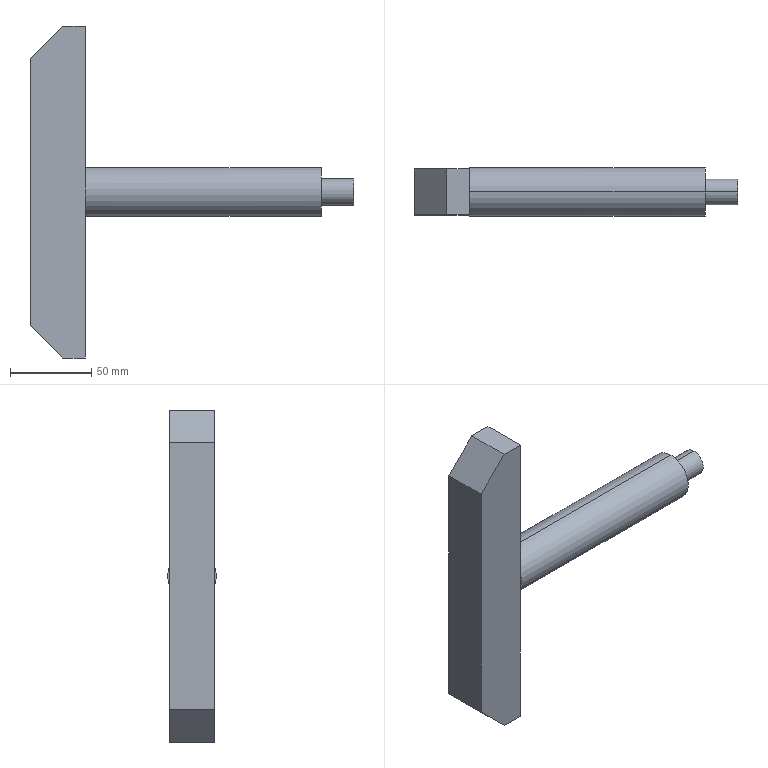Part | SolidWorks | features Chamfer 1, ICE 1, Revolution 1 | 1 solid | 17 faces | box 199 x 30 x 204 mm | volume 289524 mm3 | plane 13 | cylinder 4 | commonest cylinder face diameters 16 x2 30 x2
STEP:
#1=CARTESIAN_POINT('',(165.,0.,8.));
#2=VERTEX_POINT('',#1);
#3=CARTESIAN_POINT('',(165.,0.,-8.));
#4=VERTEX_POINT('',#3);
#5=CARTESIAN_POINT('',(165.,0.,0.));
#6=DIRECTION('',(-1.,0.,0.));
#7=DIRECTION('',(0.,0.,1.));
#8=AXIS2_PLACEMENT_3D('',#5,#6,#7);
#9=CIRCLE('',#8,8.);
#10=EDGE_CURVE('',#2,#4,#9,.T.);
#11=ORIENTED_EDGE('',*,*,#10,.T.);
#12=CARTESIAN_POINT('',(145.,0.,-8.));
#13=VERTEX_POINT('',#12);
#14=CARTESIAN_POINT('',(0.,0.,-8.));
#15=DIRECTION('',(-1.,0.,0.));
#16=VECTOR('',#15,1000.);
#17=LINE('',#14,#16);
#18=EDGE_CURVE('',#4,#13,#17,.T.);
#19=ORIENTED_EDGE('',*,*,#18,.T.);
#20=CARTESIAN_POINT('',(145.,0.,8.));
#21=VERTEX_POINT('',#20);
#22=CARTESIAN_POINT('',(145.,0.,0.));
#23=DIRECTION('',(-1.,0.,0.));
#24=DIRECTION('',(0.,0.,1.));
#25=AXIS2_PLACEMENT_3D('',#22,#23,#24);
#26=CIRCLE('',#25,8.);
#27=EDGE_CURVE('',#21,#13,#26,.T.);
#28=ORIENTED_EDGE('',*,*,#27,.F.);
#29=CARTESIAN_POINT('',(0.,0.,8.));
#30=DIRECTION('',(-1.,0.,0.));
#31=VECTOR('',#30,1000.);
#32=LINE('',#29,#31);
#33=EDGE_CURVE('',#2,#21,#32,.T.);
#34=ORIENTED_EDGE('',*,*,#33,.F.);
#35=EDGE_LOOP('',(#11,#19,#28,#34));
#36=FACE_OUTER_BOUND('',#35,.T.);
#37=CARTESIAN_POINT('',(0.,0.,0.));
#38=DIRECTION('',(-1.,0.,0.));
#39=DIRECTION('',(0.,0.,1.));
#40=AXIS2_PLACEMENT_3D('',#37,#38,#39);
#41=CYLINDRICAL_SURFACE('',#40,8.);
#42=ADVANCED_FACE('',(#36),#41,.T.);
#43=CARTESIAN_POINT('',(145.,0.,15.));
#44=VERTEX_POINT('',#43);
#45=CARTESIAN_POINT('',(145.,0.,-15.));
#46=VERTEX_POINT('',#45);
#47=CARTESIAN_POINT('',(145.,0.,0.));
#48=DIRECTION('',(-1.,0.,0.));
#49=DIRECTION('',(0.,0.,1.));
#50=AXIS2_PLACEMENT_3D('',#47,#48,#49);
#51=CIRCLE('',#50,15.);
#52=EDGE_CURVE('',#44,#46,#51,.T.);
#53=ORIENTED_EDGE('',*,*,#52,.T.);
#54=CARTESIAN_POINT('',(0.,0.,-15.));
#55=VERTEX_POINT('',#54);
#56=CARTESIAN_POINT('',(0.,0.,-15.));
#57=DIRECTION('',(-1.,0.,0.));
#58=VECTOR('',#57,1000.);
#59=LINE('',#56,#58);
#60=EDGE_CURVE('',#46,#55,#59,.T.);
#61=ORIENTED_EDGE('',*,*,#60,.T.);
#62=CARTESIAN_POINT('',(0.,14.,-5.385));
#63=VERTEX_POINT('',#62);
#64=CARTESIAN_POINT('',(0.,0.,0.));
#65=DIRECTION('',(-1.,0.,0.));
#66=DIRECTION('',(0.,0.,1.));
#67=AXIS2_PLACEMENT_3D('',#64,#65,#66);
#68=CIRCLE('',#67,15.);
#69=EDGE_CURVE('',#63,#55,#68,.T.);
#70=ORIENTED_EDGE('',*,*,#69,.F.);
#71=CARTESIAN_POINT('',(0.,14.,5.385));
#72=VERTEX_POINT('',#71);
#73=CARTESIAN_POINT('',(0.,0.,0.));
#74=DIRECTION('',(-1.,0.,0.));
#75=DIRECTION('',(0.,0.,1.));
#76=AXIS2_PLACEMENT_3D('',#73,#74,#75);
#77=CIRCLE('',#76,15.);
#78=EDGE_CURVE('',#72,#63,#77,.T.);
#79=ORIENTED_EDGE('',*,*,#78,.F.);
#80=CARTESIAN_POINT('',(0.,0.,15.));
#81=VERTEX_POINT('',#80);
#82=CARTESIAN_POINT('',(0.,0.,0.));
#83=DIRECTION('',(-1.,0.,0.));
#84=DIRECTION('',(0.,0.,1.));
#85=AXIS2_PLACEMENT_3D('',#82,#83,#84);
#86=CIRCLE('',#85,15.);
#87=EDGE_CURVE('',#81,#72,#86,.T.);
#88=ORIENTED_EDGE('',*,*,#87,.F.);
#89=CARTESIAN_POINT('',(0.,0.,15.));
#90=DIRECTION('',(-1.,0.,0.));
#91=VECTOR('',#90,1000.);
#92=LINE('',#89,#91);
#93=EDGE_CURVE('',#44,#81,#92,.T.);
#94=ORIENTED_EDGE('',*,*,#93,.F.);
#95=EDGE_LOOP('',(#53,#61,#70,#79,#88,#94));
#96=FACE_OUTER_BOUND('',#95,.T.);
#97=CARTESIAN_POINT('',(0.,0.,0.));
#98=DIRECTION('',(-1.,0.,0.));
#99=DIRECTION('',(0.,0.,1.));
#100=AXIS2_PLACEMENT_3D('',#97,#98,#99);
#101=CYLINDRICAL_SURFACE('',#100,15.);
#102=ADVANCED_FACE('',(#96),#101,.T.);
#103=CARTESIAN_POINT('',(0.,14.,102.));
#104=DIRECTION('',(0.,0.,-1.));
#105=VECTOR('',#104,1000.);
#106=LINE('',#103,#105);
#107=EDGE_CURVE('',#72,#63,#106,.T.);
#108=ORIENTED_EDGE('',*,*,#107,.F.);
#109=ORIENTED_EDGE('',*,*,#78,.T.);
#110=EDGE_LOOP('',(#108,#109));
#111=FACE_OUTER_BOUND('',#110,.T.);
#112=CARTESIAN_POINT('',(0.,0.,0.));
#113=DIRECTION('',(1.,0.,0.));
#114=DIRECTION('',(0.,0.,-1.));
#115=AXIS2_PLACEMENT_3D('',#112,#113,#114);
#116=PLANE('',#115);
#117=ADVANCED_FACE('',(#111),#116,.F.);
#118=CARTESIAN_POINT('',(0.,-14.,-5.385));
#119=VERTEX_POINT('',#118);
#120=CARTESIAN_POINT('',(0.,-14.,5.385));
#121=VERTEX_POINT('',#120);
#122=CARTESIAN_POINT('',(0.,-14.,102.));
#123=DIRECTION('',(0.,0.,1.));
#124=VECTOR('',#123,1000.);
#125=LINE('',#122,#124);
#126=EDGE_CURVE('',#119,#121,#125,.T.);
#127=ORIENTED_EDGE('',*,*,#126,.F.);
#128=CARTESIAN_POINT('',(0.,0.,0.));
#129=DIRECTION('',(-1.,0.,0.));
#130=DIRECTION('',(0.,0.,1.));
#131=AXIS2_PLACEMENT_3D('',#128,#129,#130);
#132=CIRCLE('',#131,15.);
#133=EDGE_CURVE('',#119,#121,#132,.T.);
#134=ORIENTED_EDGE('',*,*,#133,.T.);
#135=EDGE_LOOP('',(#127,#134));
#136=FACE_OUTER_BOUND('',#135,.T.);
#137=CARTESIAN_POINT('',(0.,0.,0.));
#138=DIRECTION('',(1.,0.,0.));
#139=DIRECTION('',(0.,0.,-1.));
#140=AXIS2_PLACEMENT_3D('',#137,#138,#139);
#141=PLANE('',#140);
#142=ADVANCED_FACE('',(#136),#141,.F.);
#143=ORIENTED_EDGE('',*,*,#60,.F.);
#144=CARTESIAN_POINT('',(145.,0.,0.));
#145=DIRECTION('',(-1.,0.,0.));
#146=DIRECTION('',(0.,0.,1.));
#147=AXIS2_PLACEMENT_3D('',#144,#145,#146);
#148=CIRCLE('',#147,15.);
#149=EDGE_CURVE('',#46,#44,#148,.T.);
#150=ORIENTED_EDGE('',*,*,#149,.T.);
#151=ORIENTED_EDGE('',*,*,#93,.T.);
#152=CARTESIAN_POINT('',(0.,0.,0.));
#153=DIRECTION('',(-1.,0.,0.));
#154=DIRECTION('',(0.,0.,1.));
#155=AXIS2_PLACEMENT_3D('',#152,#153,#154);
#156=CIRCLE('',#155,15.);
#157=EDGE_CURVE('',#121,#81,#156,.T.);
#158=ORIENTED_EDGE('',*,*,#157,.F.);
#159=ORIENTED_EDGE('',*,*,#133,.F.);
#160=CARTESIAN_POINT('',(0.,0.,0.));
#161=DIRECTION('',(-1.,0.,0.));
#162=DIRECTION('',(0.,0.,1.));
#163=AXIS2_PLACEMENT_3D('',#160,#161,#162);
#164=CIRCLE('',#163,15.);
#165=EDGE_CURVE('',#55,#119,#164,.T.);
#166=ORIENTED_EDGE('',*,*,#165,.F.);
#167=EDGE_LOOP('',(#143,#150,#151,#158,#159,#166));
#168=FACE_OUTER_BOUND('',#167,.T.);
#169=CARTESIAN_POINT('',(0.,0.,0.));
#170=DIRECTION('',(-1.,0.,0.));
#171=DIRECTION('',(0.,0.,1.));
#172=AXIS2_PLACEMENT_3D('',#169,#170,#171);
#173=CYLINDRICAL_SURFACE('',#172,15.);
#174=ADVANCED_FACE('',(#168),#173,.T.);
#175=ORIENTED_EDGE('',*,*,#52,.F.);
#176=ORIENTED_EDGE('',*,*,#149,.F.);
#177=EDGE_LOOP('',(#175,#176));
#178=FACE_OUTER_BOUND('',#177,.T.);
#179=ORIENTED_EDGE('',*,*,#27,.T.);
#180=CARTESIAN_POINT('',(145.,0.,0.));
#181=DIRECTION('',(-1.,0.,0.));
#182=DIRECTION('',(0.,0.,1.));
#183=AXIS2_PLACEMENT_3D('',#180,#181,#182);
#184=CIRCLE('',#183,8.);
#185=EDGE_CURVE('',#13,#21,#184,.T.);
#186=ORIENTED_EDGE('',*,*,#185,.T.);
#187=EDGE_LOOP('',(#179,#186));
#188=FACE_BOUND('',#187,.T.);
#189=CARTESIAN_POINT('',(145.,15.,0.));
#190=DIRECTION('',(-1.,0.,0.));
#191=DIRECTION('',(0.,0.,1.));
#192=AXIS2_PLACEMENT_3D('',#189,#190,#191);
#193=PLANE('',#192);
#194=ADVANCED_FACE('',(#178,#188),#193,.F.);
#195=ORIENTED_EDGE('',*,*,#18,.F.);
#196=CARTESIAN_POINT('',(165.,0.,0.));
#197=DIRECTION('',(-1.,0.,0.));
#198=DIRECTION('',(0.,0.,1.));
#199=AXIS2_PLACEMENT_3D('',#196,#197,#198);
#200=CIRCLE('',#199,8.);
#201=EDGE_CURVE('',#4,#2,#200,.T.);
#202=ORIENTED_EDGE('',*,*,#201,.T.);
#203=ORIENTED_EDGE('',*,*,#33,.T.);
#204=ORIENTED_EDGE('',*,*,#185,.F.);
#205=EDGE_LOOP('',(#195,#202,#203,#204));
#206=FACE_OUTER_BOUND('',#205,.T.);
#207=CARTESIAN_POINT('',(0.,0.,0.));
#208=DIRECTION('',(-1.,0.,0.));
#209=DIRECTION('',(0.,0.,1.));
#210=AXIS2_PLACEMENT_3D('',#207,#208,#209);
#211=CYLINDRICAL_SURFACE('',#210,8.);
#212=ADVANCED_FACE('',(#206),#211,.T.);
#213=ORIENTED_EDGE('',*,*,#10,.F.);
#214=ORIENTED_EDGE('',*,*,#201,.F.);
#215=EDGE_LOOP('',(#213,#214));
#216=FACE_OUTER_BOUND('',#215,.T.);
#217=CARTESIAN_POINT('',(165.,8.,0.));
#218=DIRECTION('',(-1.,0.,0.));
#219=DIRECTION('',(0.,0.,1.));
#220=AXIS2_PLACEMENT_3D('',#217,#218,#219);
#221=PLANE('',#220);
#222=ADVANCED_FACE('',(#216),#221,.F.);
#223=CARTESIAN_POINT('',(0.,14.,-102.));
#224=VERTEX_POINT('',#223);
#225=CARTESIAN_POINT('',(0.,14.,102.));
#226=DIRECTION('',(0.,0.,-1.));
#227=VECTOR('',#226,1000.);
#228=LINE('',#225,#227);
#229=EDGE_CURVE('',#63,#224,#228,.T.);
#230=ORIENTED_EDGE('',*,*,#229,.F.);
#231=ORIENTED_EDGE('',*,*,#69,.T.);
#232=ORIENTED_EDGE('',*,*,#165,.T.);
#233=CARTESIAN_POINT('',(0.,-14.,-102.));
#234=VERTEX_POINT('',#233);
#235=CARTESIAN_POINT('',(0.,-14.,102.));
#236=DIRECTION('',(0.,0.,1.));
#237=VECTOR('',#236,1000.);
#238=LINE('',#235,#237);
#239=EDGE_CURVE('',#234,#119,#238,.T.);
#240=ORIENTED_EDGE('',*,*,#239,.F.);
#241=CARTESIAN_POINT('',(0.,-14.,-102.));
#242=DIRECTION('',(0.,-1.,0.));
#243=VECTOR('',#242,1000.);
#244=LINE('',#241,#243);
#245=EDGE_CURVE('',#224,#234,#244,.T.);
#246=ORIENTED_EDGE('',*,*,#245,.F.);
#247=EDGE_LOOP('',(#230,#231,#232,#240,#246));
#248=FACE_OUTER_BOUND('',#247,.T.);
#249=CARTESIAN_POINT('',(0.,0.,0.));
#250=DIRECTION('',(-1.,0.,0.));
#251=DIRECTION('',(0.,0.,1.));
#252=AXIS2_PLACEMENT_3D('',#249,#250,#251);
#253=PLANE('',#252);
#254=ADVANCED_FACE('',(#248),#253,.F.);
#255=CARTESIAN_POINT('',(0.,-14.,102.));
#256=VERTEX_POINT('',#255);
#257=CARTESIAN_POINT('',(0.,-14.,102.));
#258=DIRECTION('',(0.,0.,1.));
#259=VECTOR('',#258,1000.);
#260=LINE('',#257,#259);
#261=EDGE_CURVE('',#121,#256,#260,.T.);
#262=ORIENTED_EDGE('',*,*,#261,.F.);
#263=ORIENTED_EDGE('',*,*,#157,.T.);
#264=ORIENTED_EDGE('',*,*,#87,.T.);
#265=CARTESIAN_POINT('',(0.,14.,102.));
#266=VERTEX_POINT('',#265);
#267=CARTESIAN_POINT('',(0.,14.,102.));
#268=DIRECTION('',(0.,0.,-1.));
#269=VECTOR('',#268,1000.);
#270=LINE('',#267,#269);
#271=EDGE_CURVE('',#266,#72,#270,.T.);
#272=ORIENTED_EDGE('',*,*,#271,.F.);
#273=CARTESIAN_POINT('',(0.,-14.,102.));
#274=DIRECTION('',(0.,1.,0.));
#275=VECTOR('',#274,1000.);
#276=LINE('',#273,#275);
#277=EDGE_CURVE('',#256,#266,#276,.T.);
#278=ORIENTED_EDGE('',*,*,#277,.F.);
#279=EDGE_LOOP('',(#262,#263,#264,#272,#278));
#280=FACE_OUTER_BOUND('',#279,.T.);
#281=CARTESIAN_POINT('',(0.,0.,0.));
#282=DIRECTION('',(-1.,0.,0.));
#283=DIRECTION('',(0.,0.,1.));
#284=AXIS2_PLACEMENT_3D('',#281,#282,#283);
#285=PLANE('',#284);
#286=ADVANCED_FACE('',(#280),#285,.F.);
#287=CARTESIAN_POINT('',(-14.,-14.,-102.));
#288=VERTEX_POINT('',#287);
#289=CARTESIAN_POINT('',(-34.,-14.,-102.));
#290=DIRECTION('',(1.,0.,0.));
#291=VECTOR('',#290,1000.);
#292=LINE('',#289,#291);
#293=EDGE_CURVE('',#288,#234,#292,.T.);
#294=ORIENTED_EDGE('',*,*,#293,.F.);
#295=CARTESIAN_POINT('',(-14.,14.,-102.));
#296=VERTEX_POINT('',#295);
#297=CARTESIAN_POINT('',(-14.,14.,-102.));
#298=DIRECTION('',(0.,1.,0.));
#299=VECTOR('',#298,1000.);
#300=LINE('',#297,#299);
#301=EDGE_CURVE('',#288,#296,#300,.T.);
#302=ORIENTED_EDGE('',*,*,#301,.T.);
#303=CARTESIAN_POINT('',(-34.,14.,-102.));
#304=DIRECTION('',(1.,0.,0.));
#305=VECTOR('',#304,1000.);
#306=LINE('',#303,#305);
#307=EDGE_CURVE('',#296,#224,#306,.T.);
#308=ORIENTED_EDGE('',*,*,#307,.T.);
#309=ORIENTED_EDGE('',*,*,#245,.T.);
#310=EDGE_LOOP('',(#294,#302,#308,#309));
#311=FACE_OUTER_BOUND('',#310,.T.);
#312=CARTESIAN_POINT('',(-34.,-14.,-102.));
#313=DIRECTION('',(0.,0.,1.));
#314=DIRECTION('',(1.,0.,0.));
#315=AXIS2_PLACEMENT_3D('',#312,#313,#314);
#316=PLANE('',#315);
#317=ADVANCED_FACE('',(#311),#316,.F.);
#318=CARTESIAN_POINT('',(-14.,-14.,102.));
#319=VERTEX_POINT('',#318);
#320=CARTESIAN_POINT('',(-34.,-14.,102.));
#321=DIRECTION('',(1.,0.,0.));
#322=VECTOR('',#321,1000.);
#323=LINE('',#320,#322);
#324=EDGE_CURVE('',#319,#256,#323,.T.);
#325=ORIENTED_EDGE('',*,*,#324,.F.);
#326=CARTESIAN_POINT('',(-34.,-14.,82.));
#327=VERTEX_POINT('',#326);
#328=CARTESIAN_POINT('',(-34.,-14.,82.));
#329=DIRECTION('',(-0.7071,0.,-0.7071));
#330=VECTOR('',#329,1000.);
#331=LINE('',#328,#330);
#332=EDGE_CURVE('',#319,#327,#331,.T.);
#333=ORIENTED_EDGE('',*,*,#332,.T.);
#334=CARTESIAN_POINT('',(-34.,-14.,-82.));
#335=VERTEX_POINT('',#334);
#336=CARTESIAN_POINT('',(-34.,-14.,102.));
#337=DIRECTION('',(0.,0.,1.));
#338=VECTOR('',#337,1000.);
#339=LINE('',#336,#338);
#340=EDGE_CURVE('',#335,#327,#339,.T.);
#341=ORIENTED_EDGE('',*,*,#340,.F.);
#342=CARTESIAN_POINT('',(-34.,-14.,-82.));
#343=DIRECTION('',(0.7071,0.,-0.7071));
#344=VECTOR('',#343,1000.);
#345=LINE('',#342,#344);
#346=EDGE_CURVE('',#335,#288,#345,.T.);
#347=ORIENTED_EDGE('',*,*,#346,.T.);
#348=ORIENTED_EDGE('',*,*,#293,.T.);
#349=ORIENTED_EDGE('',*,*,#239,.T.);
#350=ORIENTED_EDGE('',*,*,#126,.T.);
#351=ORIENTED_EDGE('',*,*,#261,.T.);
#352=EDGE_LOOP('',(#325,#333,#341,#347,#348,#349,#350,#351));
#353=FACE_OUTER_BOUND('',#352,.T.);
#354=CARTESIAN_POINT('',(-34.,-14.,102.));
#355=DIRECTION('',(0.,1.,0.));
#356=DIRECTION('',(0.,0.,1.));
#357=AXIS2_PLACEMENT_3D('',#354,#355,#356);
#358=PLANE('',#357);
#359=ADVANCED_FACE('',(#353),#358,.F.);
#360=CARTESIAN_POINT('',(-14.,14.,102.));
#361=VERTEX_POINT('',#360);
#362=CARTESIAN_POINT('',(-34.,14.,102.));
#363=DIRECTION('',(1.,0.,0.));
#364=VECTOR('',#363,1000.);
#365=LINE('',#362,#364);
#366=EDGE_CURVE('',#361,#266,#365,.T.);
#367=ORIENTED_EDGE('',*,*,#366,.F.);
#368=CARTESIAN_POINT('',(-14.,-14.,102.));
#369=DIRECTION('',(0.,-1.,0.));
#370=VECTOR('',#369,1000.);
#371=LINE('',#368,#370);
#372=EDGE_CURVE('',#361,#319,#371,.T.);
#373=ORIENTED_EDGE('',*,*,#372,.T.);
#374=ORIENTED_EDGE('',*,*,#324,.T.);
#375=ORIENTED_EDGE('',*,*,#277,.T.);
#376=EDGE_LOOP('',(#367,#373,#374,#375));
#377=FACE_OUTER_BOUND('',#376,.T.);
#378=CARTESIAN_POINT('',(-34.,-14.,102.));
#379=DIRECTION('',(0.,0.,-1.));
#380=DIRECTION('',(-1.,0.,0.));
#381=AXIS2_PLACEMENT_3D('',#378,#379,#380);
#382=PLANE('',#381);
#383=ADVANCED_FACE('',(#377),#382,.F.);
#384=CARTESIAN_POINT('',(-34.,14.,82.));
#385=VERTEX_POINT('',#384);
#386=CARTESIAN_POINT('',(-34.,14.,-82.));
#387=VERTEX_POINT('',#386);
#388=CARTESIAN_POINT('',(-34.,14.,102.));
#389=DIRECTION('',(0.,0.,-1.));
#390=VECTOR('',#389,1000.);
#391=LINE('',#388,#390);
#392=EDGE_CURVE('',#385,#387,#391,.T.);
#393=ORIENTED_EDGE('',*,*,#392,.F.);
#394=CARTESIAN_POINT('',(-34.,14.,82.));
#395=DIRECTION('',(0.7071,0.,0.7071));
#396=VECTOR('',#395,1000.);
#397=LINE('',#394,#396);
#398=EDGE_CURVE('',#385,#361,#397,.T.);
#399=ORIENTED_EDGE('',*,*,#398,.T.);
#400=ORIENTED_EDGE('',*,*,#366,.T.);
#401=ORIENTED_EDGE('',*,*,#271,.T.);
#402=ORIENTED_EDGE('',*,*,#107,.T.);
#403=ORIENTED_EDGE('',*,*,#229,.T.);
#404=ORIENTED_EDGE('',*,*,#307,.F.);
#405=CARTESIAN_POINT('',(-34.,14.,-82.));
#406=DIRECTION('',(-0.7071,0.,0.7071));
#407=VECTOR('',#406,1000.);
#408=LINE('',#405,#407);
#409=EDGE_CURVE('',#296,#387,#408,.T.);
#410=ORIENTED_EDGE('',*,*,#409,.T.);
#411=EDGE_LOOP('',(#393,#399,#400,#401,#402,#403,#404,#410));
#412=FACE_OUTER_BOUND('',#411,.T.);
#413=CARTESIAN_POINT('',(-34.,14.,102.));
#414=DIRECTION('',(0.,-1.,0.));
#415=DIRECTION('',(0.,0.,-1.));
#416=AXIS2_PLACEMENT_3D('',#413,#414,#415);
#417=PLANE('',#416);
#418=ADVANCED_FACE('',(#412),#417,.F.);
#419=ORIENTED_EDGE('',*,*,#340,.T.);
#420=CARTESIAN_POINT('',(-34.,14.,82.));
#421=DIRECTION('',(0.,1.,0.));
#422=VECTOR('',#421,1000.);
#423=LINE('',#420,#422);
#424=EDGE_CURVE('',#327,#385,#423,.T.);
#425=ORIENTED_EDGE('',*,*,#424,.T.);
#426=ORIENTED_EDGE('',*,*,#392,.T.);
#427=CARTESIAN_POINT('',(-34.,-14.,-82.));
#428=DIRECTION('',(0.,-1.,0.));
#429=VECTOR('',#428,1000.);
#430=LINE('',#427,#429);
#431=EDGE_CURVE('',#387,#335,#430,.T.);
#432=ORIENTED_EDGE('',*,*,#431,.T.);
#433=EDGE_LOOP('',(#419,#425,#426,#432));
#434=FACE_OUTER_BOUND('',#433,.T.);
#435=CARTESIAN_POINT('',(-34.,0.,0.));
#436=DIRECTION('',(-1.,0.,0.));
#437=DIRECTION('',(0.,0.,1.));
#438=AXIS2_PLACEMENT_3D('',#435,#436,#437);
#439=PLANE('',#438);
#440=ADVANCED_FACE('',(#434),#439,.T.);
#441=ORIENTED_EDGE('',*,*,#332,.F.);
#442=ORIENTED_EDGE('',*,*,#372,.F.);
#443=ORIENTED_EDGE('',*,*,#398,.F.);
#444=ORIENTED_EDGE('',*,*,#424,.F.);
#445=EDGE_LOOP('',(#441,#442,#443,#444));
#446=FACE_OUTER_BOUND('',#445,.T.);
#447=CARTESIAN_POINT('',(-34.,0.,82.));
#448=DIRECTION('',(-0.7071,0.,0.7071));
#449=DIRECTION('',(0.,-1.,0.));
#450=AXIS2_PLACEMENT_3D('',#447,#448,#449);
#451=PLANE('',#450);
#452=ADVANCED_FACE('',(#446),#451,.T.);
#453=ORIENTED_EDGE('',*,*,#409,.F.);
#454=ORIENTED_EDGE('',*,*,#301,.F.);
#455=ORIENTED_EDGE('',*,*,#346,.F.);
#456=ORIENTED_EDGE('',*,*,#431,.F.);
#457=EDGE_LOOP('',(#453,#454,#455,#456));
#458=FACE_OUTER_BOUND('',#457,.T.);
#459=CARTESIAN_POINT('',(-34.,0.,-82.));
#460=DIRECTION('',(-0.7071,0.,-0.7071));
#461=DIRECTION('',(0.,1.,0.));
#462=AXIS2_PLACEMENT_3D('',#459,#460,#461);
#463=PLANE('',#462);
#464=ADVANCED_FACE('',(#458),#463,.T.);
#465=CLOSED_SHELL('',(#42,#102,#117,#142,#174,#194,#212,#222,#254,#286,#317,#359,#383,#418,#440,#452,#464));
#466=MANIFOLD_SOLID_BREP('',#465);
#467=CARTESIAN_POINT('',(0.,0.,0.));
#468=DIRECTION('',(0.,0.,1.));
#469=DIRECTION('',(1.,0.,0.));
#470=AXIS2_PLACEMENT_3D('',#467,#468,#469);
#471=(LENGTH_UNIT()NAMED_UNIT(*)SI_UNIT(.MILLI.,.METRE.));
#472=UNCERTAINTY_MEASURE_WITH_UNIT(LENGTH_MEASURE(0.00001),#471,'','');
#473=(NAMED_UNIT(*)PLANE_ANGLE_UNIT()SI_UNIT($,.RADIAN.));
#474=(NAMED_UNIT(*)SI_UNIT($,.STERADIAN.)SOLID_ANGLE_UNIT());
#475=(GEOMETRIC_REPRESENTATION_CONTEXT(3)GLOBAL_UNCERTAINTY_ASSIGNED_CONTEXT((#472))GLOBAL_UNIT_ASSIGNED_CONTEXT((#471,#473,#474))REPRESENTATION_CONTEXT('',''));
#476=ADVANCED_BREP_SHAPE_REPRESENTATION('',(#466,#470),#475);